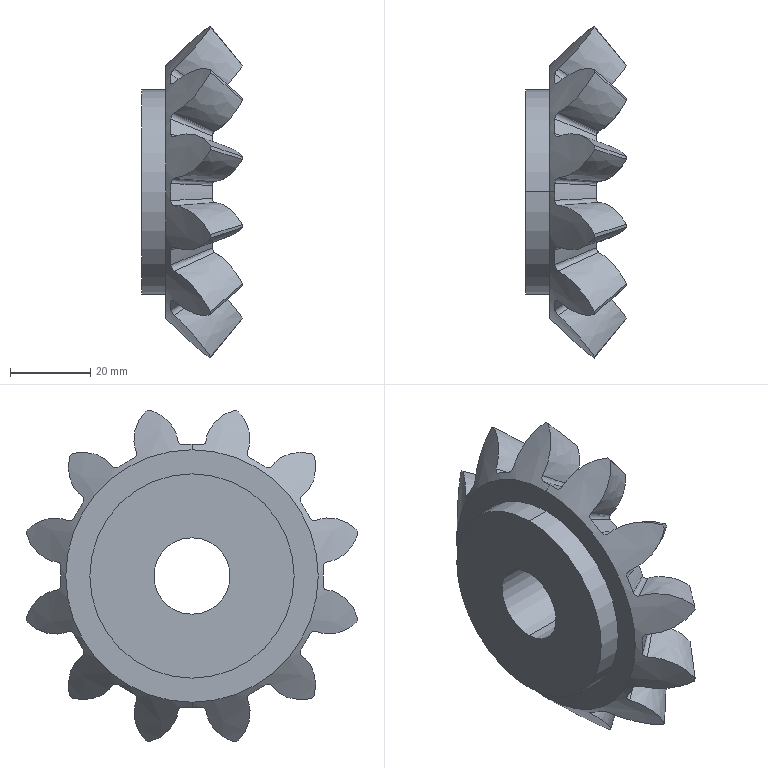Part | STEP file | straight miter gear_iso_PreviewCfg | 1 solid | 83 faces | box 25.112 x 82.518 x 82.518 mm | volume 51040 mm3 | spline 60 | cone 16 | cylinder 4 | plane 3 | commonest cylinder face diameters 19 x2 50.8 x2